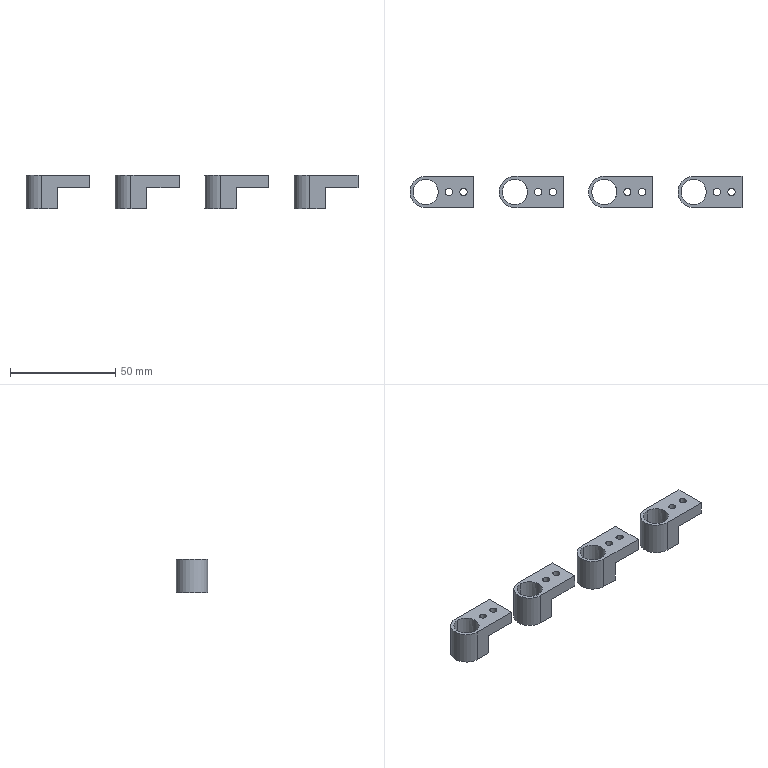NC program | NX | posted with a generic post | part box 158 x 15 x 16 mm
Lines 6060 to 6389 of 6389:
(ZLEVEL_PROFILE , TOOL : D10JING)
N12094 T14 M6
N12096 G54
N12098 G17 G0 G90 X-73.176 Y14.403 S7500 M3
N12100 G43 Z30. H14
N12102 Z-15.
N12104 G94 G1 Z-16. F1000.
N12106 X-72.366 Y13.
N12108 G3 X-71.5 Y12.5 R1.
N12110 G1 X-48.5
N12112 G2 X-43.5 Y7.5 R5.
N12114 G1 Y-7.5
N12116 G2 X-48.5 Y-12.5 R5.
N12118 G1 X-71.5
N12120 G2 X-84. Y0. R12.5
N12122 X-71.5 Y12.5 R12.5
N12124 G3 X-70.634 Y13. R1.
N12126 G1 X-69.768 Y14.5
N12128 Z-15.
N12130 G0 Z30.
N12132 X-30.676 Y14.403
N12134 Z-15.
N12136 G1 Z-16.
N12138 X-29.866 Y13.
N12140 G3 X-29. Y12.5 R1.
N12142 G1 X-6.
N12144 G2 X-1. Y7.5 R5.
N12146 G1 Y-7.5
N12148 G2 X-6. Y-12.5 R5.
N12150 G1 X-29.
N12152 G2 X-41.5 Y0. R12.5
N12154 X-29. Y12.5 R12.5
N12156 G3 X-28.134 Y13. R1.
N12158 G1 X-27.268 Y14.5
N12160 Z-15.
N12162 G0 Z30.
N12164 X11.824 Y14.403
N12166 Z-15.
N12168 G1 Z-16.
N12170 X12.634 Y13.
N12172 G3 X13.5 Y12.5 R1.
N12174 G1 X36.5
N12176 G2 X41.5 Y7.5 R5.
N12178 G1 Y-7.5
N12180 G2 X36.5 Y-12.5 R5.
N12182 G1 X13.5
N12184 G2 X1. Y0. R12.5
N12186 X13.5 Y12.5 R12.5
N12188 G3 X14.366 Y13. R1.
N12190 G1 X15.232 Y14.5
N12192 Z-15.
N12194 G0 Z30.
N12196 X54.324 Y14.403
N12198 Z-15.
N12200 G1 Z-16.
N12202 X55.134 Y13.
N12204 G3 X56. Y12.5 R1.
N12206 G1 X79.
N12208 G2 X84. Y7.5 R5.
N12210 G1 Y-7.5
N12212 G2 X79. Y-12.5 R5.
N12214 G1 X56.
N12216 G2 X43.5 Y0. R12.5
N12218 X56. Y12.5 R12.5
N12220 G3 X56.866 Y13. R1.
N12222 G1 X57.732 Y14.5
N12224 Z-15.
N12226 G0 Z30.
N12228 M5
(PLANAR_MILL , TOOL : D6A45)
N12230 T01 M6
N12232 G54
N12234 G17 G0 G90 X74.621 Y-0.383 S7500 M3
N12236 G43 Z30. H1
N12238 Z1.
N12240 G94 G1 Z-1. F1250.
N12242 G3 X74.8 Y0. R0.5
N12244 X74. Y0.8 R0.8
N12246 X74.8 Y0. R-0.8
N12248 X74.621 Y0.383 R0.5
N12250 G1 Z1.
N12252 G0 Z30.
N12254 X66.617 Y-0.621
N12256 Z1.
N12258 G1 Z-1.
N12260 G3 X67. Y-0.8 R0.5
N12262 X67.8 Y0. R0.8
N12264 X67. Y-0.8 R-0.8
N12266 X67.383 Y-0.621 R0.5
N12268 G1 Z1.
N12270 G0 Z30.
N12272 X66.734 Y8.757
N12274 Z1.
N12276 G1 Z-1.
N12278 G3 X67.5 Y8.4 R1.
N12280 G1 X79.
N12282 G2 X79.9 Y7.5 R0.9
N12284 G1 Y-7.5
N12286 G2 X79. Y-8.4 R0.9
N12288 G1 X56.
N12290 G2 X47.6 Y0. R8.4
N12292 X56. Y8.4 R8.4
N12294 G1 X67.5
N12296 G3 X68.266 Y8.757 R1.
N12298 G1 Z1.
N12300 G0 Z30.
N12302 X56.766 Y4.743
N12304 Z1.
N12306 G1 Z-1.
N12308 G3 X56. Y5.1 R1.
N12310 X50.9 Y0. R5.1
N12312 X56. Y5.1 R-5.1
N12314 X55.234 Y4.743 R1.
N12316 G1 Z1.
N12318 G0 Z30.
N12320 X31.883 Y0.621
N12322 Z1.
N12324 G1 Z-1.
N12326 G3 X31.5 Y0.8 R0.5
N12328 X30.7 Y0. R0.8
N12330 X31.5 Y0.8 R-0.8
N12332 X31.117 Y0.621 R0.5
N12334 G1 Z1.
N12336 G0 Z30.
N12338 X24.883
N12340 Z1.
N12342 G1 Z-1.
N12344 G3 X24.5 Y0.8 R0.5
N12346 X23.7 Y0. R0.8
N12348 X24.5 Y0.8 R-0.8
N12350 X24.117 Y0.621 R0.5
N12352 G1 Z1.
N12354 G0 Z30.
N12356 X24.234 Y8.757
N12358 Z1.
N12360 G1 Z-1.
N12362 G3 X25. Y8.4 R1.
N12364 G1 X36.5
N12366 G2 X37.4 Y7.5 R0.9
N12368 G1 Y-7.5
N12370 G2 X36.5 Y-8.4 R0.9
N12372 G1 X13.5
N12374 G2 X5.1 Y0. R8.4
N12376 X13.5 Y8.4 R8.4
N12378 G1 X25.
N12380 G3 X25.766 Y8.757 R1.
N12382 G1 Z1.
N12384 G0 Z30.
N12386 X14.266 Y4.743
N12388 Z1.
N12390 G1 Z-1.
N12392 G3 X13.5 Y5.1 R1.
N12394 X8.4 Y0. R5.1
N12396 X13.5 Y5.1 R-5.1
N12398 X12.734 Y4.743 R1.
N12400 G1 Z1.
N12402 G0 Z30.
N12404 X-11.383 Y-0.621
N12406 Z1.
N12408 G1 Z-1.
N12410 G3 X-11. Y-0.8 R0.5
N12412 X-10.2 Y0. R0.8
N12414 X-11. Y-0.8 R-0.8
N12416 X-10.617 Y-0.621 R0.5
N12418 G1 Z1.
N12420 G0 Z30.
N12422 X-18.383
N12424 Z1.
N12426 G1 Z-1.
N12428 G3 X-18. Y-0.8 R0.5
N12430 X-17.2 Y0. R0.8
N12432 X-18. Y-0.8 R-0.8
N12434 X-17.617 Y-0.621 R0.5
N12436 G1 Z1.
N12438 G0 Z30.
N12440 X-18.266 Y8.757
N12442 Z1.
N12444 G1 Z-1.
N12446 G3 X-17.5 Y8.4 R1.
N12448 G1 X-6.
N12450 G2 X-5.1 Y7.5 R0.9
N12452 G1 Y-7.5
N12454 G2 X-6. Y-8.4 R0.9
N12456 G1 X-29.
N12458 G2 X-37.4 Y0. R8.4
N12460 X-29. Y8.4 R8.4
N12462 G1 X-17.5
N12464 G3 X-16.734 Y8.757 R1.
N12466 G1 Z1.
N12468 G0 Z30.
N12470 X-28.234 Y4.743
N12472 Z1.
N12474 G1 Z-1.
N12476 G3 X-29. Y5.1 R1.
N12478 X-34.1 Y0. R5.1
N12480 X-29. Y5.1 R-5.1
N12482 X-29.766 Y4.743 R1.
N12484 G1 Z1.
N12486 G0 Z30.
N12488 X-53.117 Y0.621
N12490 Z1.
N12492 G1 Z-1.
N12494 G3 X-53.5 Y0.8 R0.5
N12496 X-54.3 Y0. R0.8
N12498 X-53.5 Y0.8 R-0.8
N12500 X-53.883 Y0.621 R0.5
N12502 G1 Z1.
N12504 G0 Z30.
N12506 X-60.883 Y-0.621
N12508 Z1.
N12510 G1 Z-1.
N12512 G3 X-60.5 Y-0.8 R0.5
N12514 X-59.7 Y0. R0.8
N12516 X-60.5 Y-0.8 R-0.8
N12518 X-60.117 Y-0.621 R0.5
N12520 G1 Z1.
N12522 G0 Z30.
N12524 X-60.766 Y8.757
N12526 Z1.
N12528 G1 Z-1.
N12530 G3 X-60. Y8.4 R1.
N12532 G1 X-48.5
N12534 G2 X-47.6 Y7.5 R0.9
N12536 G1 Y-7.5
N12538 G2 X-48.5 Y-8.4 R0.9
N12540 G1 X-71.5
N12542 G2 X-79.9 Y0. R8.4
N12544 X-71.5 Y8.4 R8.4
N12546 G1 X-60.
N12548 G3 X-59.234 Y8.757 R1.
N12550 G1 Z1.
N12552 G0 Z30.
N12554 X-70.734 Y4.743
N12556 Z1.
N12558 G1 Z-1.
N12560 G3 X-71.5 Y5.1 R1.
N12562 X-76.6 Y0. R5.1
N12564 X-71.5 Y5.1 R-5.1
N12566 X-72.266 Y4.743 R1.
N12568 G1 Z1.
N12570 G0 Z30.
N12572 M5
(刀补14 , TOOL : D10JING)
N12574 T14 M6
N12576 G54
N12578 G17 G0 G90 X-71.5 Y0. S7500 M3
N12580 G43 Z30. H14
N12582 Z0.5
N12584 G41 G94 G1 X-71.496 Y-0.1 F1000. D14
N12586 G3 X-70.55 Y0. R0.478
N12588 X-70.55 Y0. Z-1.5 I-0.95 J0.
N12590 X-70.55 Y0. Z-3.5 I-0.95 J0.
N12592 X-70.55 Y0. Z-5.5 I-0.95 J0.
N12594 X-70.55 Y0. Z-7.5 I-0.95 J0.
N12596 X-70.55 Y0. Z-9.5 I-0.95 J0.
N12598 X-70.55 Y0. Z-11.5 I-0.95 J0.
N12600 X-70.55 Y0. Z-13.5 I-0.95 J0.
N12602 X-70.55 Y0. Z-15.5 I-0.95 J0.
N12604 X-71.5 Y0.95 Z-16. R0.95
N12606 X-72.45 Y0. R0.95
N12608 X-71.5 Y0.95 R-0.95
N12610 X-71.6 Y0.004 R0.478
N12612 G40
N12614 G1 X-71.5 Y0.
N12616 G0 Z30.
N12618 X-29.
N12620 Z0.5
N12622 G41 G1 X-28.996 Y-0.1
N12624 G3 X-28.05 Y0. R0.478
N12626 X-28.05 Y0. Z-1.5 I-0.95 J0.
N12628 X-28.05 Y0. Z-3.5 I-0.95 J0.
N12630 X-28.05 Y0. Z-5.5 I-0.95 J0.
N12632 X-28.05 Y0. Z-7.5 I-0.95 J0.
N12634 X-28.05 Y0. Z-9.5 I-0.95 J0.
N12636 X-28.05 Y0. Z-11.5 I-0.95 J0.
N12638 X-28.05 Y0. Z-13.5 I-0.95 J0.
N12640 X-28.05 Y0. Z-15.5 I-0.95 J0.
N12642 X-29. Y0.95 Z-16. R0.95
N12644 X-29.95 Y0. R0.95
N12646 X-29. Y0.95 R-0.95
N12648 X-29.1 Y0.004 R0.478
N12650 G40
N12652 G1 X-29. Y0.
N12654 G0 Z30.
N12656 X13.5
N12658 Z0.5
N12660 G41 G1 X13.504 Y-0.1
N12662 G3 X14.45 Y0. R0.478
N12664 X14.45 Y0. Z-1.5 I-0.95 J0.
N12666 X14.45 Y0. Z-3.5 I-0.95 J0.
N12668 X14.45 Y0. Z-5.5 I-0.95 J0.
N12670 X14.45 Y0. Z-7.5 I-0.95 J0.
N12672 X14.45 Y0. Z-9.5 I-0.95 J0.
N12674 X14.45 Y0. Z-11.5 I-0.95 J0.
N12676 X14.45 Y0. Z-13.5 I-0.95 J0.
N12678 X14.45 Y0. Z-15.5 I-0.95 J0.
N12680 X13.5 Y0.95 Z-16. R0.95
N12682 X12.55 Y0. R0.95
N12684 X13.5 Y0.95 R-0.95
N12686 X13.4 Y0.004 R0.478
N12688 G40
N12690 G1 X13.5 Y0.
N12692 G0 Z30.
N12694 X56.
N12696 Z0.5
N12698 G41 G1 X56.004 Y-0.1
N12700 G3 X56.95 Y0. R0.478
N12702 X56.95 Y0. Z-1.5 I-0.95 J0.
N12704 X56.95 Y0. Z-3.5 I-0.95 J0.
N12706 X56.95 Y0. Z-5.5 I-0.95 J0.
N12708 X56.95 Y0. Z-7.5 I-0.95 J0.
N12710 X56.95 Y0. Z-9.5 I-0.95 J0.
N12712 X56.95 Y0. Z-11.5 I-0.95 J0.
N12714 X56.95 Y0. Z-13.5 I-0.95 J0.
N12716 X56.95 Y0. Z-15.5 I-0.95 J0.
N12718 X56. Y0.95 Z-16. R0.95
N12720 X55.05 Y0. R0.95
N12722 X56. Y0.95 R-0.95
N12724 X55.9 Y0.004 R0.478
N12726 G40
N12728 G1 X56. Y0.
N12730 G0 Z30.
N12732 M5
N12734 M2